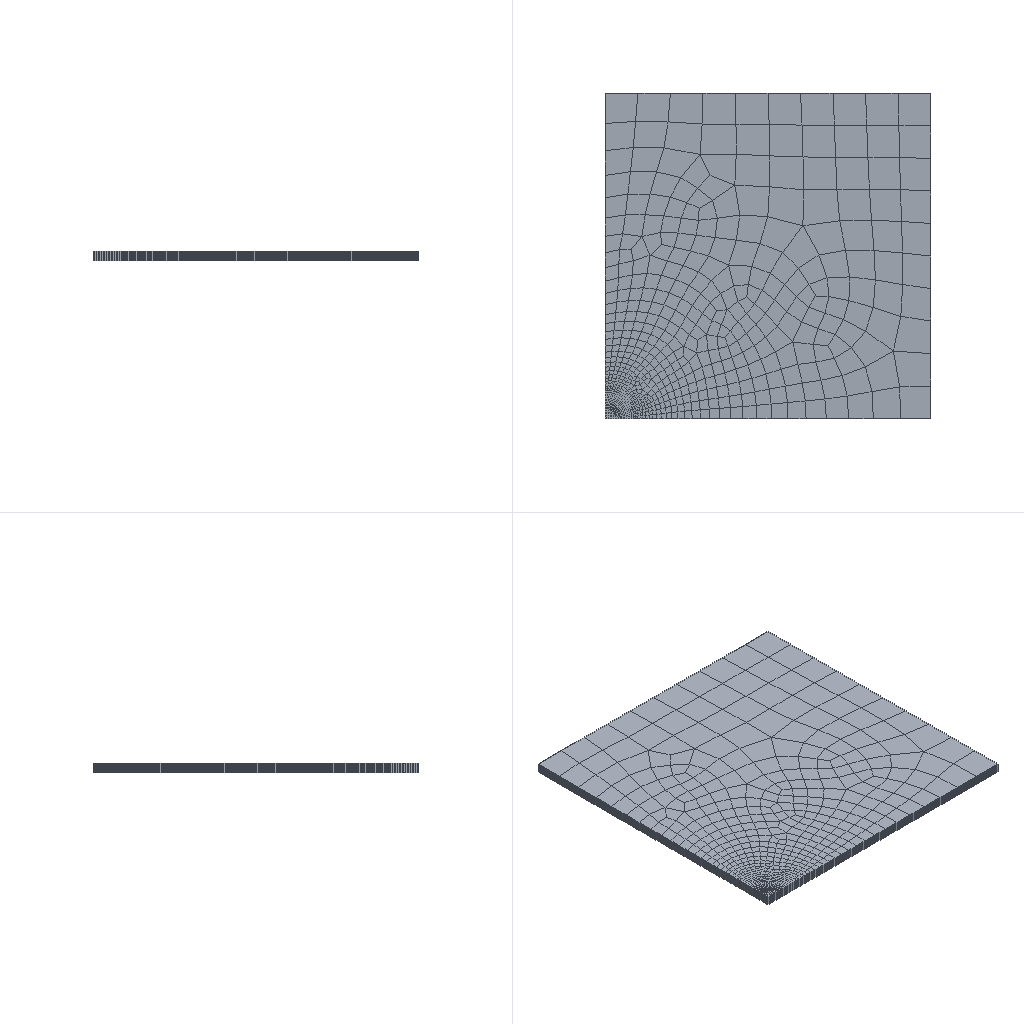Simulation study | abaqus
Set-up summary:
category,name,step,type,value,unit,region
solver,abaqus,,Abaqus/CAE 2024
units,mm-N-s-tonne (MPa),,inferred,E= density=1.78e-09
analysis,Step-1,,dynamic explicit,nlgeom=True; time_period=0.002
mesh,nodes,,,17095
mesh,elements,,,15161
element_type,C3D8R,,,15160
element_type,MASS,,,1
material,Mat-T700,,density,1.78e-09
material,Mat-T700,,behaviors,depvar; user material
section,Mat-T700,,solid section,,,_I1
section,Mat-T700,,solid section,,,_I2
section,Mat-T700,,solid section,,,_I3
section,Mat-T700,,solid section,,,_I4
load,Predefined,initial,initial condition velocity
bc,BC-P,initial,pinned,[dofs=PINNED],,_PickedSet37
bc,BC-RP,initial,fixed,"[dofs=rx,ry,rz,x,y n=5]",,Set-RP
bc,BC-X,initial,xsymm,[dofs=XSYMM],,_PickedSet35
bc,BC-Y,initial,ysymm,[dofs=YSYMM],,_PickedSet36
contact,Int-1,Step-1,contact pair,interaction=IntProp-1,,Punch-1.Surf-1 / Set-Nds_CNS_
constraint,rigid body,,,1
Abaqus input file, long lists of numbers shortened:
*Heading
** Job name: deck Model name: Model-1
** Generated by: Abaqus/CAE 2024
*Preprint, echo=NO, model=NO, history=NO, contact=NO
**
** PARTS
**
*Part, name=Lam-C
*Node
    815,           0.,           7.,           0.
    816,           7.,           0.,           0.
** (17092 more lines like these left out)
*Element, type=C3D8R
 759,  831,  832,  964,  972, 1645, 1646, 1778, 1786
 760,  855,  982,  980,  854, 1669, 1796, 1794, 1668
** (15158 more lines like these left out)
*Elset, elset=C-Layer-1, generate
  759,  1516,     1
*Elset, elset=C-Layer-2, generate
 1517,  2274,     1
*Elset, elset=C-Layer-3, generate
 2275,  3032,     1
*Elset, elset=C-Layer-4, generate
 3033,  3790,     1
*Elset, elset=C-Layer-5, generate
 3791,  4548,     1
*Elset, elset=C-Layer-6, generate
 4549,  5306,     1
*Elset, elset=C-Layer-7, generate
 5307,  6064,     1
*Elset, elset=C-Layer-8, generate
 6065,  6822,     1
*Elset, elset=C-Layer-9, generate
 6823,  7580,     1
*Elset, elset=C-Layer-10, generate
 7581,  8338,     1
*Elset, elset=C-Layer-11, generate
 8339,  9096,     1
*Elset, elset=C-Layer-12, generate
 9097,  9854,     1
*Elset, elset=C-Layer-13, generate
  9855,  10612,      1
*Elset, elset=C-Layer-14, generate
 10613,  11370,      1
*Elset, elset=C-Layer-15, generate
 11371,  12128,      1
*Elset, elset=C-Layer-16, generate
 12129,  12886,      1
*Elset, elset=C-Layer-17, generate
 12887,  13644,      1
*Elset, elset=C-Layer-18, generate
 13645,  14402,      1
*Elset, elset=C-Layer-19, generate
 14403,  15160,      1
*Elset, elset=C-Layer-20, generate
 15161,  15918,      1
*Elset, elset=_PickedSet23, internal, generate
   759,  15918,      1
*Orientation, name=Ori-1
          1.,           0.,           0.,           0.,           1.,           0.
3, 0.
** Region: (Sect-T700:Picked), (Controls:EC-1), (Material Orientation:Picked)
*Elset, elset=_I1, internal
   759,   760,   761,   762,   763,   764,   765,   766,   767,   768,   769,   770,   771,   772,   773,   774
   775,   776,   777,   778,   779,   780,   781,   782,   783,   784,   785,   786,   787,   788,   789,   790
** (235 more lines like these left out)
** Section: Sect-T700
*Solid Section, elset=_I1, orientation=Ori-1, controls=EC-1, material=Mat-T700
,
*Orientation, name=Ori-2
          1.,           0.,           0.,           0.,           1.,           0.
3, 45.
** Region: (Sect-T700:Picked), (Controls:EC-1), (Material Orientation:Picked)
*Elset, elset=_I2, internal
  1517,  1518,  1519,  1520,  1521,  1522,  1523,  1524,  1525,  1526,  1527,  1528,  1529,  1530,  1531,  1532
  1533,  1534,  1535,  1536,  1537,  1538,  1539,  1540,  1541,  1542,  1543,  1544,  1545,  1546,  1547,  1548
** (235 more lines like these left out)
** Section: Sect-T700
*Solid Section, elset=_I2, orientation=Ori-2, controls=EC-1, material=Mat-T700
,
*Orientation, name=Ori-3
          1.,           0.,           0.,           0.,           1.,           0.
3, -45.
** Region: (Sect-T700:Picked), (Controls:EC-1), (Material Orientation:Picked)
*Elset, elset=_I3, internal
  2275,  2276,  2277,  2278,  2279,  2280,  2281,  2282,  2283,  2284,  2285,  2286,  2287,  2288,  2289,  2290
  2291,  2292,  2293,  2294,  2295,  2296,  2297,  2298,  2299,  2300,  2301,  2302,  2303,  2304,  2305,  2306
** (235 more lines like these left out)
** Section: Sect-T700
*Solid Section, elset=_I3, orientation=Ori-3, controls=EC-1, material=Mat-T700
,
*Orientation, name=Ori-4
          1.,           0.,           0.,           0.,           1.,           0.
3, 90.
** Region: (Sect-T700:Picked), (Controls:EC-1), (Material Orientation:Picked)
*Elset, elset=_I4, internal
  3033,  3034,  3035,  3036,  3037,  3038,  3039,  3040,  3041,  3042,  3043,  3044,  3045,  3046,  3047,  3048
  3049,  3050,  3051,  3052,  3053,  3054,  3055,  3056,  3057,  3058,  3059,  3060,  3061,  3062,  3063,  3064
** (235 more lines like these left out)
** Section: Sect-T700
*Solid Section, elset=_I4, orientation=Ori-4, controls=EC-1, material=Mat-T700
,
*End Part
**
*Part, name=Punch
*End Part
**
**
** ASSEMBLY
**
*Assembly, name=Assembly
**
*Instance, name=Lam-C-1, part=Lam-C
*End Instance
**
*Instance, name=Punch-1, part=Punch
          0.,           0.,         8.01
          0.,           0.,         8.01, 1.,           0.,         8.01, 90.
*Node
      1,           0.,           0.,           0.
*Nset, nset=Punch-1-RefPt_, internal
1,
*Nset, nset=_PickedSet3, internal
 1,
*Surface, type=REVOLUTION, name=Surf-1
START,           5.,           0.
 CIRCL,           0.,          -5.,           0.,           0.
*Rigid Body, ref node=Punch-1-RefPt_, analytical surface=Surf-1
*Element, type=MASS, elset=_PickedSet3_Inertia-1_
1, 1
*Mass, elset=_PickedSet3_Inertia-1_
0.0001,
*End Instance
**
*Nset, nset=Set-Nds, instance=Lam-C-1
   820,   821,   822,   920,   921,   922,   923,   924,   925,   926,   927,   928,   929,   930,   931,   932
   933,   934,   935,   936,   937,   938,   939,   940,   943,   944,   945,   946,   947,   948,   949,   950
** (240 more lines like these left out)
*Nset, nset=Set-RP, instance=Punch-1
 1,
*Nset, nset=_PickedSet35, internal, instance=Lam-C-1
   815,   819,   820,   822,   890,   891,   892,   893,   894,   895,   896,   897,   898,   899,   900,   901
   902,   903,   904,   905,   906,   907,   908,   909,   910,   911,   912,   913,   914,   915,   916,   917
** (59 more lines like these left out)
*Nset, nset=_PickedSet36, internal, instance=Lam-C-1
   816,   817,   821,   822,   842,   843,   844,   845,   846,   847,   848,   849,   850,   851,   852,   853
   854,   855,   856,   857,   858,   859,   860,   861,   862,   863,   864,   865,   866,   867,   868,   869
** (59 more lines like these left out)
*Nset, nset=_PickedSet37, internal, instance=Lam-C-1
   817,   818,   819,   872,   873,   874,   875,   876,   877,   878,   879,   880,   881,   882,   883,   884
   885,   886,   887,   888,   889,  1631,  1632,  1633,  1686,  1687,  1688,  1689,  1690,  1691,  1692,  1693
** (26 more lines like these left out)
*Surface, type=NODE, name=Set-Nds_CNS_, internal
Set-Nds, 1.
*End Assembly
**
** ELEMENT CONTROLS
**
*Section Controls, name=EC-1, ELEMENT DELETION=YES, hourglass=RELAX STIFFNESS
1., 1., 1.
**
** MATERIALS
**
*Material, name=Mat-T700
*Density
 1.78e-09,
*Depvar, delete=8
      8,
*User Material, constants=14
114000.,8610.,  0.3, 0.45,4160.,3000.,2688.,1458.
 69.5, 236., 55.5, 175., 136., 95.6
**
** INTERACTION PROPERTIES
**
*Surface Interaction, name=IntProp-1
**
** BOUNDARY CONDITIONS
**
** Name: BC-P Type: Symmetry/Antisymmetry/Encastre
*Boundary
_PickedSet37, PINNED
** Name: BC-RP Type: Displacement/Rotation
*Boundary
Set-RP, 1, 1
Set-RP, 2, 2
Set-RP, 4, 4
Set-RP, 5, 5
Set-RP, 6, 6
** Name: BC-X Type: Symmetry/Antisymmetry/Encastre
*Boundary
_PickedSet35, XSYMM
** Name: BC-Y Type: Symmetry/Antisymmetry/Encastre
*Boundary
_PickedSet36, YSYMM
**
** PREDEFINED FIELDS
**
** Name: Predefined Field-1   Type: Velocity
*Initial Conditions, type=VELOCITY
Set-RP, 1, 0.
Set-RP, 2, 0.
Set-RP, 3, -5000.
** ----------------------------------------------------------------
**
** STEP: Step-1
**
*Step, name=Step-1, nlgeom=YES
*Dynamic, Explicit
, 0.002
*Bulk Viscosity
0.06, 1.2
**
** INTERACTIONS
**
** Interaction: Int-1
*Contact Pair, interaction=IntProp-1, mechanical constraint=KINEMATIC, cpset=Int-1
Punch-1.Surf-1, Set-Nds_CNS_
**
** OUTPUT REQUESTS
**
*Restart, write, number interval=1, time marks=NO
**
** FIELD OUTPUT: F-Output-1
**
*Output, field, number interval=100
*Node Output
U,
*Element Output, directions=YES
E, S, SDV, STATUS
**
** HISTORY OUTPUT: H-Output-1
**
*Output, history, time interval=2e-05
*Node Output, nset=Set-RP
A3, U3, V3
*End Step
Results summary:
result,odb.job_status,,,JOB_STATUS_COMPLETED_SUCCESSFULLY,"consistent, unstated (Abaqus has no unit system)"
result,steps[0].procedure,Step-1,,"*DYNAMIC, EXPLICIT","consistent, unstated (Abaqus has no unit system)"
result,steps[0].time_period,Step-1,,0.002,"consistent, unstated (Abaqus has no unit system)"
result,steps[0].n_frames,Step-1,,101,"consistent, unstated (Abaqus has no unit system)"
result,steps[0].last_frame.id,Step-1,,182807,"consistent, unstated (Abaqus has no unit system)"
result,steps[0].last_frame.value,Step-1,,0.002,"consistent, unstated (Abaqus has no unit system)"
result,steps[0].last_frame.description,Step-1,,Increment    182807: Step Time =   2.0000E-03,"consistent, unstated (Abaqus has no unit system)"
result,steps[0].completed,Step-1,,True,"consistent, unstated (Abaqus has no unit system)"
result,steps[0].max_U_magnitude,Step-1,,193.537,"consistent, unstated (Abaqus has no unit system)"
result,steps[0].max_S_mises,Step-1,,60.333,"consistent, unstated (Abaqus has no unit system)"
result,steps[0].diagnostic.n_increments,Step-1,,101,"consistent, unstated (Abaqus has no unit system)"